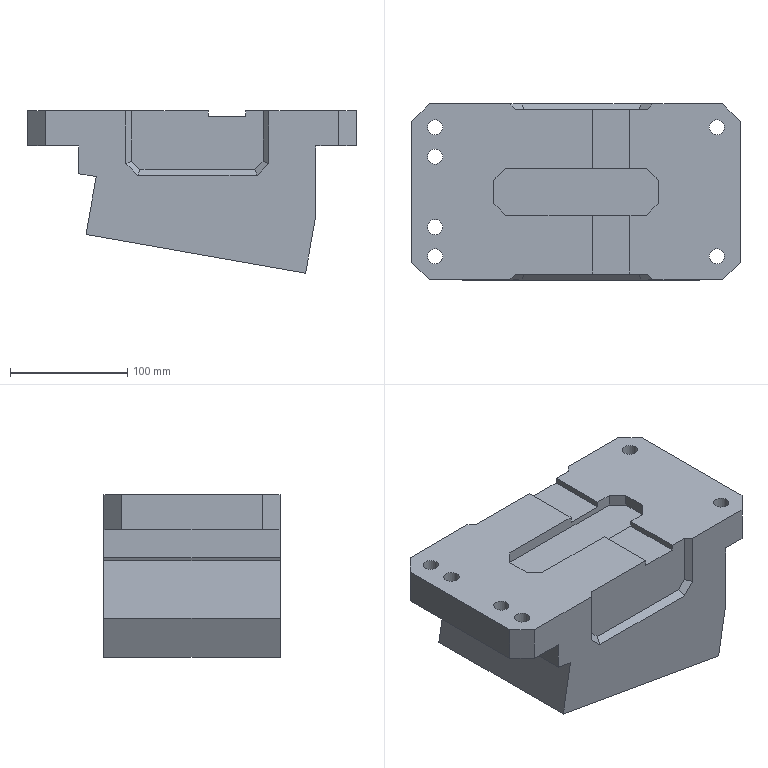Part | NX | features solid 2 | 1 solid | 59 faces | box 280 x 150 x 138.395 mm | volume 3767128 mm3 | plane 49 | cylinder 10 | commonest cylinder face diameters 13 x6 20 x4